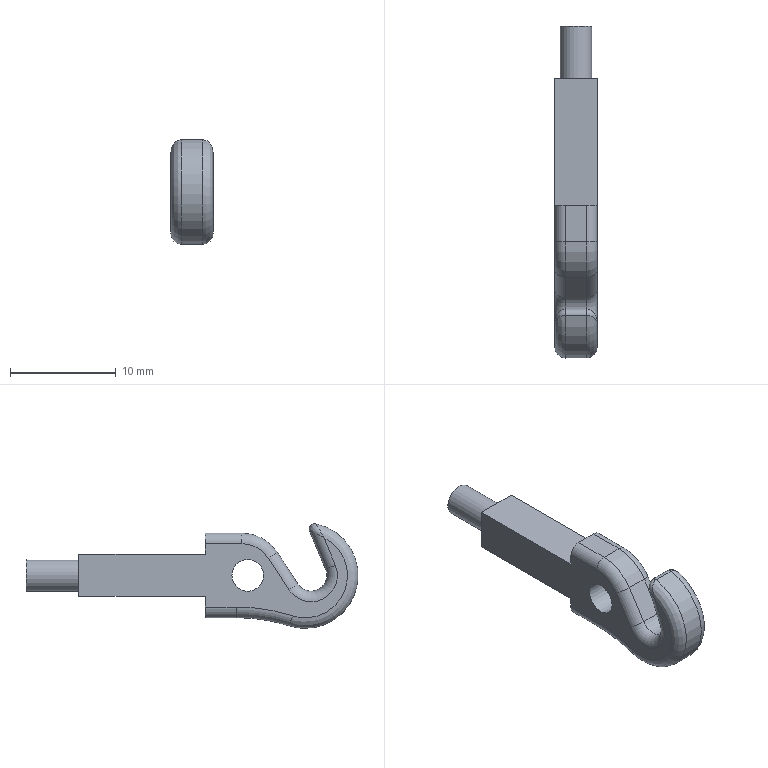Part | STEP file | 1-30.1 | 1 solid | 37 faces | box 4 x 31.452 x 9.916 mm | volume 569.945 mm3 | cylinder 14 | plane 12 | spline 6 | torus 5 | commonest cylinder face diameters 2 x8 3 x3 1 x1 8 x1 33 x1